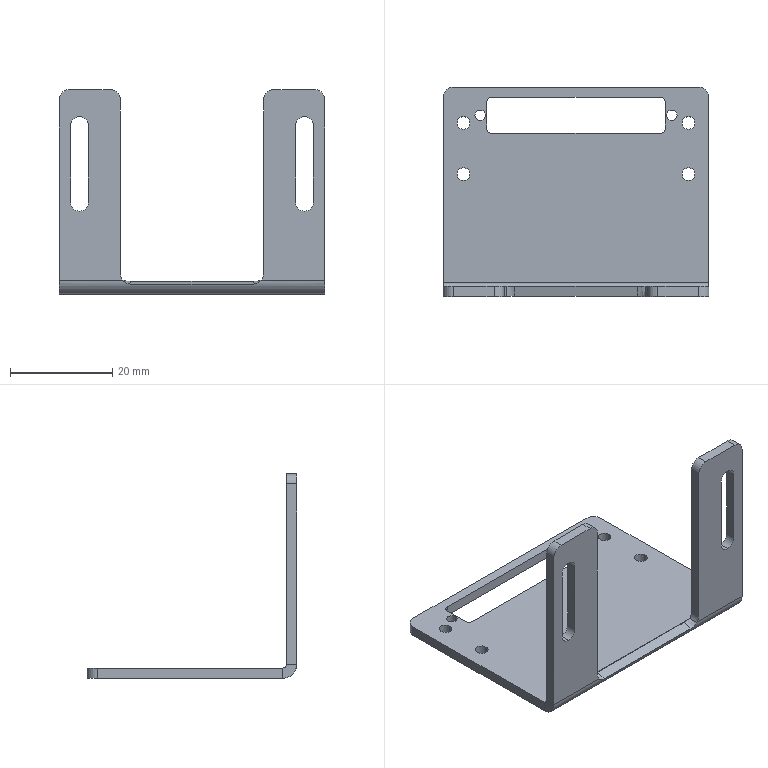Part | STEP file | 06-01-05 light source mounting plate A (Default) | 1 solid | 60 faces | box 52 x 41 x 40 mm | volume 5228 mm3 | cylinder 32 | plane 26 | spline 2 | commonest cylinder face diameters 2.5 x8 4 x8 3.5 x6 2 x4 2.05 x4 1.473 x1